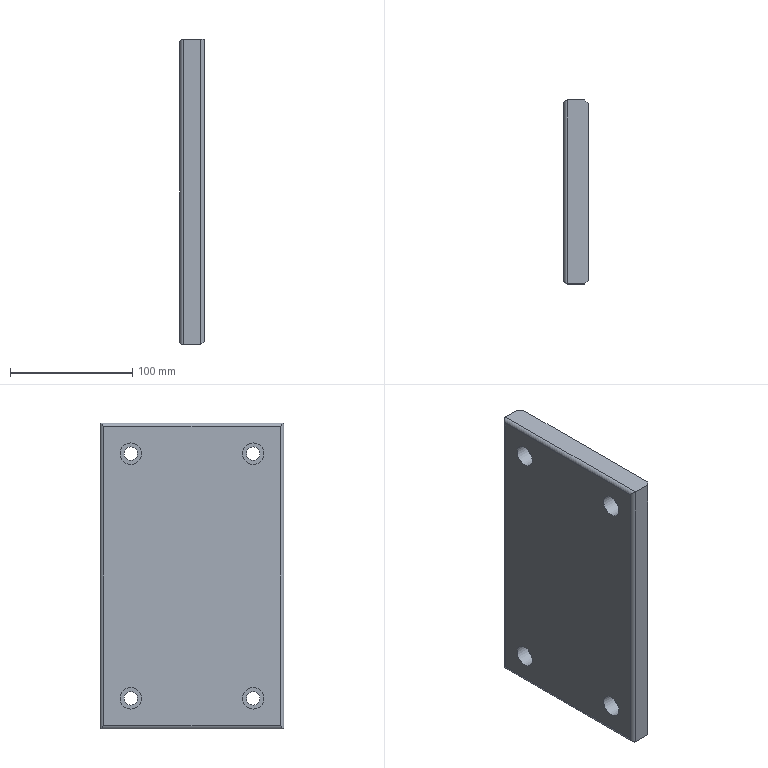Part | NX | features solid 2 | 1 solid | 25 faces | box 20 x 150 x 250 mm | volume 730972 mm3 | plane 13 | cylinder 12 | commonest cylinder face diameters 6 x4 11 x4 17.5 x4
STEP:
#1=CARTESIAN_POINT('',(-1123.,1070.,-255.));
#2=VERTEX_POINT('',#1);
#3=CARTESIAN_POINT('',(-1137.,1070.,-255.));
#4=VERTEX_POINT('',#3);
#5=CARTESIAN_POINT('',(-1120.,1070.,-255.));
#6=DIRECTION('',(-1.,0.,0.));
#7=VECTOR('',#6,1000.);
#8=LINE('',#5,#7);
#9=EDGE_CURVE('',#2,#4,#8,.T.);
#10=ORIENTED_EDGE('',*,*,#9,.F.);
#11=CARTESIAN_POINT('',(-1123.,920.,-255.));
#12=VERTEX_POINT('',#11);
#13=CARTESIAN_POINT('',(-1123.,920.,-255.));
#14=DIRECTION('',(0.,-1.,0.));
#15=VECTOR('',#14,1000.);
#16=LINE('',#13,#15);
#17=EDGE_CURVE('',#2,#12,#16,.T.);
#18=ORIENTED_EDGE('',*,*,#17,.T.);
#19=CARTESIAN_POINT('',(-1137.,920.,-255.));
#20=VERTEX_POINT('',#19);
#21=CARTESIAN_POINT('',(-1120.,920.,-255.));
#22=DIRECTION('',(-1.,0.,0.));
#23=VECTOR('',#22,1000.);
#24=LINE('',#21,#23);
#25=EDGE_CURVE('',#12,#20,#24,.T.);
#26=ORIENTED_EDGE('',*,*,#25,.T.);
#27=CARTESIAN_POINT('',(-1137.,1070.,-255.));
#28=DIRECTION('',(0.,1.,0.));
#29=VECTOR('',#28,1000.);
#30=LINE('',#27,#29);
#31=EDGE_CURVE('',#20,#4,#30,.T.);
#32=ORIENTED_EDGE('',*,*,#31,.T.);
#33=EDGE_LOOP('',(#10,#18,#26,#32));
#34=FACE_BOUND('',#33,.T.);
#35=CARTESIAN_POINT('',(-1120.,920.,-255.));
#36=DIRECTION('',(0.,0.,1.));
#37=DIRECTION('',(0.,-1.,0.));
#38=AXIS2_PLACEMENT_3D('',#35,#36,#37);
#39=PLANE('',#38);
#40=ADVANCED_FACE('',(#34),#39,.F.);
#41=CARTESIAN_POINT('',(-1123.,1070.,-5.));
#42=VERTEX_POINT('',#41);
#43=CARTESIAN_POINT('',(-1137.,1070.,-5.));
#44=VERTEX_POINT('',#43);
#45=CARTESIAN_POINT('',(-1120.,1070.,-5.));
#46=DIRECTION('',(-1.,0.,0.));
#47=VECTOR('',#46,1000.);
#48=LINE('',#45,#47);
#49=EDGE_CURVE('',#42,#44,#48,.T.);
#50=ORIENTED_EDGE('',*,*,#49,.F.);
#51=CARTESIAN_POINT('',(-1123.,1070.,-205.));
#52=DIRECTION('',(0.,0.,-1.));
#53=VECTOR('',#52,1000.);
#54=LINE('',#51,#53);
#55=EDGE_CURVE('',#42,#2,#54,.T.);
#56=ORIENTED_EDGE('',*,*,#55,.T.);
#57=ORIENTED_EDGE('',*,*,#9,.T.);
#58=CARTESIAN_POINT('',(-1137.,1070.,-5.));
#59=DIRECTION('',(0.,0.,1.));
#60=VECTOR('',#59,1000.);
#61=LINE('',#58,#60);
#62=EDGE_CURVE('',#4,#44,#61,.T.);
#63=ORIENTED_EDGE('',*,*,#62,.T.);
#64=EDGE_LOOP('',(#50,#56,#57,#63));
#65=FACE_BOUND('',#64,.T.);
#66=CARTESIAN_POINT('',(-1120.,1070.,-205.));
#67=DIRECTION('',(0.,-1.,0.));
#68=DIRECTION('',(1.,0.,0.));
#69=AXIS2_PLACEMENT_3D('',#66,#67,#68);
#70=PLANE('',#69);
#71=ADVANCED_FACE('',(#65),#70,.F.);
#72=CARTESIAN_POINT('',(-1123.,920.,-5.));
#73=VERTEX_POINT('',#72);
#74=CARTESIAN_POINT('',(-1137.,920.,-5.));
#75=VERTEX_POINT('',#74);
#76=CARTESIAN_POINT('',(-1120.,920.,-5.));
#77=DIRECTION('',(-1.,0.,0.));
#78=VECTOR('',#77,1000.);
#79=LINE('',#76,#78);
#80=EDGE_CURVE('',#73,#75,#79,.T.);
#81=ORIENTED_EDGE('',*,*,#80,.F.);
#82=CARTESIAN_POINT('',(-1120.,923.,-5.));
#83=VERTEX_POINT('',#82);
#84=CARTESIAN_POINT('',(-1120.,923.,-5.));
#85=DIRECTION('',(0.7071,0.7071,0.));
#86=VECTOR('',#85,1000.);
#87=LINE('',#84,#86);
#88=EDGE_CURVE('',#73,#83,#87,.T.);
#89=ORIENTED_EDGE('',*,*,#88,.T.);
#90=CARTESIAN_POINT('',(-1120.,1067.,-5.));
#91=VERTEX_POINT('',#90);
#92=CARTESIAN_POINT('',(-1120.,1070.,-5.));
#93=DIRECTION('',(0.,-1.,0.));
#94=VECTOR('',#93,1000.);
#95=LINE('',#92,#94);
#96=EDGE_CURVE('',#91,#83,#95,.T.);
#97=ORIENTED_EDGE('',*,*,#96,.F.);
#98=CARTESIAN_POINT('',(-1120.,1067.,-5.));
#99=DIRECTION('',(-0.7071,0.7071,0.));
#100=VECTOR('',#99,1000.);
#101=LINE('',#98,#100);
#102=EDGE_CURVE('',#91,#42,#101,.T.);
#103=ORIENTED_EDGE('',*,*,#102,.T.);
#104=ORIENTED_EDGE('',*,*,#49,.T.);
#105=CARTESIAN_POINT('',(-1137.,920.,-5.));
#106=DIRECTION('',(0.,-1.,0.));
#107=VECTOR('',#106,1000.);
#108=LINE('',#105,#107);
#109=EDGE_CURVE('',#44,#75,#108,.T.);
#110=ORIENTED_EDGE('',*,*,#109,.T.);
#111=EDGE_LOOP('',(#81,#89,#97,#103,#104,#110));
#112=FACE_BOUND('',#111,.T.);
#113=CARTESIAN_POINT('',(-1120.,1070.,-5.));
#114=DIRECTION('',(0.,0.,-1.));
#115=DIRECTION('',(1.,0.,0.));
#116=AXIS2_PLACEMENT_3D('',#113,#114,#115);
#117=PLANE('',#116);
#118=ADVANCED_FACE('',(#112),#117,.F.);
#119=ORIENTED_EDGE('',*,*,#25,.F.);
#120=CARTESIAN_POINT('',(-1123.,920.,-5.));
#121=DIRECTION('',(0.,0.,1.));
#122=VECTOR('',#121,1000.);
#123=LINE('',#120,#122);
#124=EDGE_CURVE('',#12,#73,#123,.T.);
#125=ORIENTED_EDGE('',*,*,#124,.T.);
#126=ORIENTED_EDGE('',*,*,#80,.T.);
#127=CARTESIAN_POINT('',(-1137.,920.,-205.));
#128=DIRECTION('',(0.,0.,-1.));
#129=VECTOR('',#128,1000.);
#130=LINE('',#127,#129);
#131=EDGE_CURVE('',#75,#20,#130,.T.);
#132=ORIENTED_EDGE('',*,*,#131,.T.);
#133=EDGE_LOOP('',(#119,#125,#126,#132));
#134=FACE_BOUND('',#133,.T.);
#135=CARTESIAN_POINT('',(-1120.,920.,-5.));
#136=DIRECTION('',(0.,1.,0.));
#137=DIRECTION('',(0.,0.,1.));
#138=AXIS2_PLACEMENT_3D('',#135,#136,#137);
#139=PLANE('',#138);
#140=ADVANCED_FACE('',(#134),#139,.F.);
#141=CARTESIAN_POINT('',(-1120.,1067.,-252.));
#142=VERTEX_POINT('',#141);
#143=CARTESIAN_POINT('',(-1120.,1067.,-205.));
#144=DIRECTION('',(0.,0.,1.));
#145=VECTOR('',#144,1000.);
#146=LINE('',#143,#145);
#147=EDGE_CURVE('',#142,#91,#146,.T.);
#148=ORIENTED_EDGE('',*,*,#147,.T.);
#149=ORIENTED_EDGE('',*,*,#96,.T.);
#150=CARTESIAN_POINT('',(-1120.,923.,-252.));
#151=VERTEX_POINT('',#150);
#152=CARTESIAN_POINT('',(-1120.,923.,-205.));
#153=DIRECTION('',(0.,0.,-1.));
#154=VECTOR('',#153,1000.);
#155=LINE('',#152,#154);
#156=EDGE_CURVE('',#83,#151,#155,.T.);
#157=ORIENTED_EDGE('',*,*,#156,.T.);
#158=CARTESIAN_POINT('',(-1120.,920.,-252.));
#159=DIRECTION('',(0.,1.,0.));
#160=VECTOR('',#159,1000.);
#161=LINE('',#158,#160);
#162=EDGE_CURVE('',#151,#142,#161,.T.);
#163=ORIENTED_EDGE('',*,*,#162,.T.);
#164=EDGE_LOOP('',(#148,#149,#157,#163));
#165=FACE_BOUND('',#164,.T.);
#166=CARTESIAN_POINT('',(-1120.,1045.,-35.5));
#167=VERTEX_POINT('',#166);
#168=CARTESIAN_POINT('',(-1120.,1045.,-30.));
#169=DIRECTION('',(-1.,0.,0.));
#170=DIRECTION('',(0.,0.,-1.));
#171=AXIS2_PLACEMENT_3D('',#168,#169,#170);
#172=CIRCLE('',#171,5.5);
#173=EDGE_CURVE('',#167,#167,#172,.T.);
#174=ORIENTED_EDGE('',*,*,#173,.T.);
#175=EDGE_LOOP('',(#174));
#176=FACE_BOUND('',#175,.T.);
#177=CARTESIAN_POINT('',(-1120.,945.,-35.5));
#178=VERTEX_POINT('',#177);
#179=CARTESIAN_POINT('',(-1120.,945.,-30.));
#180=DIRECTION('',(-1.,0.,0.));
#181=DIRECTION('',(0.,0.,-1.));
#182=AXIS2_PLACEMENT_3D('',#179,#180,#181);
#183=CIRCLE('',#182,5.5);
#184=EDGE_CURVE('',#178,#178,#183,.T.);
#185=ORIENTED_EDGE('',*,*,#184,.T.);
#186=EDGE_LOOP('',(#185));
#187=FACE_BOUND('',#186,.T.);
#188=CARTESIAN_POINT('',(-1120.,1045.,-235.5));
#189=VERTEX_POINT('',#188);
#190=CARTESIAN_POINT('',(-1120.,1045.,-230.));
#191=DIRECTION('',(-1.,0.,0.));
#192=DIRECTION('',(0.,0.,-1.));
#193=AXIS2_PLACEMENT_3D('',#190,#191,#192);
#194=CIRCLE('',#193,5.5);
#195=EDGE_CURVE('',#189,#189,#194,.T.);
#196=ORIENTED_EDGE('',*,*,#195,.T.);
#197=EDGE_LOOP('',(#196));
#198=FACE_BOUND('',#197,.T.);
#199=CARTESIAN_POINT('',(-1120.,945.,-235.5));
#200=VERTEX_POINT('',#199);
#201=CARTESIAN_POINT('',(-1120.,945.,-230.));
#202=DIRECTION('',(-1.,0.,0.));
#203=DIRECTION('',(0.,0.,-1.));
#204=AXIS2_PLACEMENT_3D('',#201,#202,#203);
#205=CIRCLE('',#204,5.5);
#206=EDGE_CURVE('',#200,#200,#205,.T.);
#207=ORIENTED_EDGE('',*,*,#206,.T.);
#208=EDGE_LOOP('',(#207));
#209=FACE_BOUND('',#208,.T.);
#210=CARTESIAN_POINT('',(-1120.,920.,-205.));
#211=DIRECTION('',(-1.,0.,0.));
#212=DIRECTION('',(0.,0.,-1.));
#213=AXIS2_PLACEMENT_3D('',#210,#211,#212);
#214=PLANE('',#213);
#215=ADVANCED_FACE('',(#165,#176,#187,#198,#209),#214,.F.);
#216=CARTESIAN_POINT('',(-1140.,1067.,-252.));
#217=VERTEX_POINT('',#216);
#218=CARTESIAN_POINT('',(-1140.,923.,-252.));
#219=VERTEX_POINT('',#218);
#220=CARTESIAN_POINT('',(-1140.,920.,-252.));
#221=DIRECTION('',(0.,1.,0.));
#222=VECTOR('',#221,1000.);
#223=LINE('',#220,#222);
#224=EDGE_CURVE('',#217,#219,#223,.F.);
#225=ORIENTED_EDGE('',*,*,#224,.T.);
#226=CARTESIAN_POINT('',(-1140.,923.,-8.));
#227=VERTEX_POINT('',#226);
#228=CARTESIAN_POINT('',(-1140.,923.,-5.));
#229=DIRECTION('',(0.,0.,-1.));
#230=VECTOR('',#229,1000.);
#231=LINE('',#228,#230);
#232=EDGE_CURVE('',#219,#227,#231,.F.);
#233=ORIENTED_EDGE('',*,*,#232,.T.);
#234=CARTESIAN_POINT('',(-1140.,1067.,-8.));
#235=VERTEX_POINT('',#234);
#236=CARTESIAN_POINT('',(-1140.,1070.,-8.));
#237=DIRECTION('',(0.,-1.,0.));
#238=VECTOR('',#237,1000.);
#239=LINE('',#236,#238);
#240=EDGE_CURVE('',#227,#235,#239,.F.);
#241=ORIENTED_EDGE('',*,*,#240,.T.);
#242=CARTESIAN_POINT('',(-1140.,1067.,-205.));
#243=DIRECTION('',(0.,0.,1.));
#244=VECTOR('',#243,1000.);
#245=LINE('',#242,#244);
#246=EDGE_CURVE('',#235,#217,#245,.F.);
#247=ORIENTED_EDGE('',*,*,#246,.T.);
#248=EDGE_LOOP('',(#225,#233,#241,#247));
#249=FACE_BOUND('',#248,.T.);
#250=CARTESIAN_POINT('',(-1140.,1045.,-21.25));
#251=VERTEX_POINT('',#250);
#252=CARTESIAN_POINT('',(-1140.,1045.,-30.));
#253=DIRECTION('',(1.,0.,0.));
#254=DIRECTION('',(0.,0.,1.));
#255=AXIS2_PLACEMENT_3D('',#252,#253,#254);
#256=CIRCLE('',#255,8.75);
#257=EDGE_CURVE('',#251,#251,#256,.T.);
#258=ORIENTED_EDGE('',*,*,#257,.T.);
#259=EDGE_LOOP('',(#258));
#260=FACE_BOUND('',#259,.T.);
#261=CARTESIAN_POINT('',(-1140.,945.,-21.25));
#262=VERTEX_POINT('',#261);
#263=CARTESIAN_POINT('',(-1140.,945.,-30.));
#264=DIRECTION('',(1.,0.,0.));
#265=DIRECTION('',(0.,0.,1.));
#266=AXIS2_PLACEMENT_3D('',#263,#264,#265);
#267=CIRCLE('',#266,8.75);
#268=EDGE_CURVE('',#262,#262,#267,.T.);
#269=ORIENTED_EDGE('',*,*,#268,.T.);
#270=EDGE_LOOP('',(#269));
#271=FACE_BOUND('',#270,.T.);
#272=CARTESIAN_POINT('',(-1140.,1045.,-221.25));
#273=VERTEX_POINT('',#272);
#274=CARTESIAN_POINT('',(-1140.,1045.,-230.));
#275=DIRECTION('',(1.,0.,0.));
#276=DIRECTION('',(0.,0.,1.));
#277=AXIS2_PLACEMENT_3D('',#274,#275,#276);
#278=CIRCLE('',#277,8.75);
#279=EDGE_CURVE('',#273,#273,#278,.T.);
#280=ORIENTED_EDGE('',*,*,#279,.T.);
#281=EDGE_LOOP('',(#280));
#282=FACE_BOUND('',#281,.T.);
#283=CARTESIAN_POINT('',(-1140.,945.,-221.25));
#284=VERTEX_POINT('',#283);
#285=CARTESIAN_POINT('',(-1140.,945.,-230.));
#286=DIRECTION('',(1.,0.,0.));
#287=DIRECTION('',(0.,0.,1.));
#288=AXIS2_PLACEMENT_3D('',#285,#286,#287);
#289=CIRCLE('',#288,8.75);
#290=EDGE_CURVE('',#284,#284,#289,.T.);
#291=ORIENTED_EDGE('',*,*,#290,.T.);
#292=EDGE_LOOP('',(#291));
#293=FACE_BOUND('',#292,.T.);
#294=CARTESIAN_POINT('',(-1140.,920.,-205.));
#295=DIRECTION('',(-1.,0.,0.));
#296=DIRECTION('',(0.,0.,-1.));
#297=AXIS2_PLACEMENT_3D('',#294,#295,#296);
#298=PLANE('',#297);
#299=ADVANCED_FACE('',(#249,#260,#271,#282,#293),#298,.T.);
#300=CARTESIAN_POINT('',(-1128.,945.,-224.5));
#301=VERTEX_POINT('',#300);
#302=CARTESIAN_POINT('',(-1128.,945.,-230.));
#303=DIRECTION('',(1.,0.,0.));
#304=DIRECTION('',(0.,0.,1.));
#305=AXIS2_PLACEMENT_3D('',#302,#303,#304);
#306=CIRCLE('',#305,5.5);
#307=EDGE_CURVE('',#301,#301,#306,.T.);
#308=ORIENTED_EDGE('',*,*,#307,.F.);
#309=EDGE_LOOP('',(#308));
#310=FACE_BOUND('',#309,.T.);
#311=ORIENTED_EDGE('',*,*,#206,.F.);
#312=EDGE_LOOP('',(#311));
#313=FACE_BOUND('',#312,.T.);
#314=CARTESIAN_POINT('',(-1090.,945.,-230.));
#315=DIRECTION('',(1.,0.,0.));
#316=DIRECTION('',(0.,0.,1.));
#317=AXIS2_PLACEMENT_3D('',#314,#315,#316);
#318=CYLINDRICAL_SURFACE('',#317,5.5);
#319=ADVANCED_FACE('',(#310,#313),#318,.F.);
#320=ORIENTED_EDGE('',*,*,#307,.T.);
#321=EDGE_LOOP('',(#320));
#322=FACE_BOUND('',#321,.T.);
#323=CARTESIAN_POINT('',(-1128.,945.,-221.25));
#324=VERTEX_POINT('',#323);
#325=CARTESIAN_POINT('',(-1128.,945.,-230.));
#326=DIRECTION('',(1.,0.,0.));
#327=DIRECTION('',(0.,0.,1.));
#328=AXIS2_PLACEMENT_3D('',#325,#326,#327);
#329=CIRCLE('',#328,8.75);
#330=EDGE_CURVE('',#324,#324,#329,.T.);
#331=ORIENTED_EDGE('',*,*,#330,.F.);
#332=EDGE_LOOP('',(#331));
#333=FACE_BOUND('',#332,.T.);
#334=CARTESIAN_POINT('',(-1128.,945.,-230.));
#335=DIRECTION('',(1.,0.,0.));
#336=DIRECTION('',(0.,0.,1.));
#337=AXIS2_PLACEMENT_3D('',#334,#335,#336);
#338=PLANE('',#337);
#339=ADVANCED_FACE('',(#322,#333),#338,.F.);
#340=ORIENTED_EDGE('',*,*,#330,.T.);
#341=EDGE_LOOP('',(#340));
#342=FACE_BOUND('',#341,.T.);
#343=ORIENTED_EDGE('',*,*,#290,.F.);
#344=EDGE_LOOP('',(#343));
#345=FACE_BOUND('',#344,.T.);
#346=CARTESIAN_POINT('',(-1140.,945.,-230.));
#347=DIRECTION('',(1.,0.,0.));
#348=DIRECTION('',(0.,0.,1.));
#349=AXIS2_PLACEMENT_3D('',#346,#347,#348);
#350=CYLINDRICAL_SURFACE('',#349,8.75);
#351=ADVANCED_FACE('',(#342,#345),#350,.F.);
#352=CARTESIAN_POINT('',(-1128.,1045.,-224.5));
#353=VERTEX_POINT('',#352);
#354=CARTESIAN_POINT('',(-1128.,1045.,-230.));
#355=DIRECTION('',(1.,0.,0.));
#356=DIRECTION('',(0.,0.,1.));
#357=AXIS2_PLACEMENT_3D('',#354,#355,#356);
#358=CIRCLE('',#357,5.5);
#359=EDGE_CURVE('',#353,#353,#358,.T.);
#360=ORIENTED_EDGE('',*,*,#359,.F.);
#361=EDGE_LOOP('',(#360));
#362=FACE_BOUND('',#361,.T.);
#363=ORIENTED_EDGE('',*,*,#195,.F.);
#364=EDGE_LOOP('',(#363));
#365=FACE_BOUND('',#364,.T.);
#366=CARTESIAN_POINT('',(-1090.,1045.,-230.));
#367=DIRECTION('',(1.,0.,0.));
#368=DIRECTION('',(0.,0.,1.));
#369=AXIS2_PLACEMENT_3D('',#366,#367,#368);
#370=CYLINDRICAL_SURFACE('',#369,5.5);
#371=ADVANCED_FACE('',(#362,#365),#370,.F.);
#372=ORIENTED_EDGE('',*,*,#359,.T.);
#373=EDGE_LOOP('',(#372));
#374=FACE_BOUND('',#373,.T.);
#375=CARTESIAN_POINT('',(-1128.,1045.,-221.25));
#376=VERTEX_POINT('',#375);
#377=CARTESIAN_POINT('',(-1128.,1045.,-230.));
#378=DIRECTION('',(1.,0.,0.));
#379=DIRECTION('',(0.,0.,1.));
#380=AXIS2_PLACEMENT_3D('',#377,#378,#379);
#381=CIRCLE('',#380,8.75);
#382=EDGE_CURVE('',#376,#376,#381,.T.);
#383=ORIENTED_EDGE('',*,*,#382,.F.);
#384=EDGE_LOOP('',(#383));
#385=FACE_BOUND('',#384,.T.);
#386=CARTESIAN_POINT('',(-1128.,1045.,-230.));
#387=DIRECTION('',(1.,0.,0.));
#388=DIRECTION('',(0.,0.,1.));
#389=AXIS2_PLACEMENT_3D('',#386,#387,#388);
#390=PLANE('',#389);
#391=ADVANCED_FACE('',(#374,#385),#390,.F.);
#392=ORIENTED_EDGE('',*,*,#382,.T.);
#393=EDGE_LOOP('',(#392));
#394=FACE_BOUND('',#393,.T.);
#395=ORIENTED_EDGE('',*,*,#279,.F.);
#396=EDGE_LOOP('',(#395));
#397=FACE_BOUND('',#396,.T.);
#398=CARTESIAN_POINT('',(-1140.,1045.,-230.));
#399=DIRECTION('',(1.,0.,0.));
#400=DIRECTION('',(0.,0.,1.));
#401=AXIS2_PLACEMENT_3D('',#398,#399,#400);
#402=CYLINDRICAL_SURFACE('',#401,8.75);
#403=ADVANCED_FACE('',(#394,#397),#402,.F.);
#404=CARTESIAN_POINT('',(-1128.,945.,-24.5));
#405=VERTEX_POINT('',#404);
#406=CARTESIAN_POINT('',(-1128.,945.,-30.));
#407=DIRECTION('',(1.,0.,0.));
#408=DIRECTION('',(0.,0.,1.));
#409=AXIS2_PLACEMENT_3D('',#406,#407,#408);
#410=CIRCLE('',#409,5.5);
#411=EDGE_CURVE('',#405,#405,#410,.T.);
#412=ORIENTED_EDGE('',*,*,#411,.F.);
#413=EDGE_LOOP('',(#412));
#414=FACE_BOUND('',#413,.T.);
#415=ORIENTED_EDGE('',*,*,#184,.F.);
#416=EDGE_LOOP('',(#415));
#417=FACE_BOUND('',#416,.T.);
#418=CARTESIAN_POINT('',(-1090.,945.,-30.));
#419=DIRECTION('',(1.,0.,0.));
#420=DIRECTION('',(0.,0.,1.));
#421=AXIS2_PLACEMENT_3D('',#418,#419,#420);
#422=CYLINDRICAL_SURFACE('',#421,5.5);
#423=ADVANCED_FACE('',(#414,#417),#422,.F.);
#424=ORIENTED_EDGE('',*,*,#411,.T.);
#425=EDGE_LOOP('',(#424));
#426=FACE_BOUND('',#425,.T.);
#427=CARTESIAN_POINT('',(-1128.,945.,-21.25));
#428=VERTEX_POINT('',#427);
#429=CARTESIAN_POINT('',(-1128.,945.,-30.));
#430=DIRECTION('',(1.,0.,0.));
#431=DIRECTION('',(0.,0.,1.));
#432=AXIS2_PLACEMENT_3D('',#429,#430,#431);
#433=CIRCLE('',#432,8.75);
#434=EDGE_CURVE('',#428,#428,#433,.T.);
#435=ORIENTED_EDGE('',*,*,#434,.F.);
#436=EDGE_LOOP('',(#435));
#437=FACE_BOUND('',#436,.T.);
#438=CARTESIAN_POINT('',(-1128.,945.,-30.));
#439=DIRECTION('',(1.,0.,0.));
#440=DIRECTION('',(0.,0.,1.));
#441=AXIS2_PLACEMENT_3D('',#438,#439,#440);
#442=PLANE('',#441);
#443=ADVANCED_FACE('',(#426,#437),#442,.F.);
#444=ORIENTED_EDGE('',*,*,#434,.T.);
#445=EDGE_LOOP('',(#444));
#446=FACE_BOUND('',#445,.T.);
#447=ORIENTED_EDGE('',*,*,#268,.F.);
#448=EDGE_LOOP('',(#447));
#449=FACE_BOUND('',#448,.T.);
#450=CARTESIAN_POINT('',(-1140.,945.,-30.));
#451=DIRECTION('',(1.,0.,0.));
#452=DIRECTION('',(0.,0.,1.));
#453=AXIS2_PLACEMENT_3D('',#450,#451,#452);
#454=CYLINDRICAL_SURFACE('',#453,8.75);
#455=ADVANCED_FACE('',(#446,#449),#454,.F.);
#456=CARTESIAN_POINT('',(-1128.,1045.,-24.5));
#457=VERTEX_POINT('',#456);
#458=CARTESIAN_POINT('',(-1128.,1045.,-30.));
#459=DIRECTION('',(1.,0.,0.));
#460=DIRECTION('',(0.,0.,1.));
#461=AXIS2_PLACEMENT_3D('',#458,#459,#460);
#462=CIRCLE('',#461,5.5);
#463=EDGE_CURVE('',#457,#457,#462,.T.);
#464=ORIENTED_EDGE('',*,*,#463,.F.);
#465=EDGE_LOOP('',(#464));
#466=FACE_BOUND('',#465,.T.);
#467=ORIENTED_EDGE('',*,*,#173,.F.);
#468=EDGE_LOOP('',(#467));
#469=FACE_BOUND('',#468,.T.);
#470=CARTESIAN_POINT('',(-1090.,1045.,-30.));
#471=DIRECTION('',(1.,0.,0.));
#472=DIRECTION('',(0.,0.,1.));
#473=AXIS2_PLACEMENT_3D('',#470,#471,#472);
#474=CYLINDRICAL_SURFACE('',#473,5.5);
#475=ADVANCED_FACE('',(#466,#469),#474,.F.);
#476=ORIENTED_EDGE('',*,*,#463,.T.);
#477=EDGE_LOOP('',(#476));
#478=FACE_BOUND('',#477,.T.);
#479=CARTESIAN_POINT('',(-1128.,1045.,-21.25));
#480=VERTEX_POINT('',#479);
#481=CARTESIAN_POINT('',(-1128.,1045.,-30.));
#482=DIRECTION('',(1.,0.,0.));
#483=DIRECTION('',(0.,0.,1.));
#484=AXIS2_PLACEMENT_3D('',#481,#482,#483);
#485=CIRCLE('',#484,8.75);
#486=EDGE_CURVE('',#480,#480,#485,.T.);
#487=ORIENTED_EDGE('',*,*,#486,.F.);
#488=EDGE_LOOP('',(#487));
#489=FACE_BOUND('',#488,.T.);
#490=CARTESIAN_POINT('',(-1128.,1045.,-30.));
#491=DIRECTION('',(1.,0.,0.));
#492=DIRECTION('',(0.,0.,1.));
#493=AXIS2_PLACEMENT_3D('',#490,#491,#492);
#494=PLANE('',#493);
#495=ADVANCED_FACE('',(#478,#489),#494,.F.);
#496=ORIENTED_EDGE('',*,*,#486,.T.);
#497=EDGE_LOOP('',(#496));
#498=FACE_BOUND('',#497,.T.);
#499=ORIENTED_EDGE('',*,*,#257,.F.);
#500=EDGE_LOOP('',(#499));
#501=FACE_BOUND('',#500,.T.);
#502=CARTESIAN_POINT('',(-1140.,1045.,-30.));
#503=DIRECTION('',(1.,0.,0.));
#504=DIRECTION('',(0.,0.,1.));
#505=AXIS2_PLACEMENT_3D('',#502,#503,#504);
#506=CYLINDRICAL_SURFACE('',#505,8.75);
#507=ADVANCED_FACE('',(#498,#501),#506,.F.);
#508=CARTESIAN_POINT('',(-1137.,1067.,-252.));
#509=DIRECTION('',(0.,-0.7071,-0.7071));
#510=DIRECTION('',(0.,-0.7071,0.7071));
#511=AXIS2_PLACEMENT_3D('',#508,#509,#510);
#512=ELLIPSE('',#511,4.243,3.);
#513=EDGE_CURVE('',#217,#4,#512,.T.);
#514=ORIENTED_EDGE('',*,*,#513,.F.);
#515=ORIENTED_EDGE('',*,*,#246,.F.);
#516=CARTESIAN_POINT('',(-1137.,1067.,-8.));
#517=DIRECTION('',(0.,0.7071,-0.7071));
#518=DIRECTION('',(0.,-0.7071,-0.7071));
#519=AXIS2_PLACEMENT_3D('',#516,#517,#518);
#520=ELLIPSE('',#519,4.243,3.);
#521=EDGE_CURVE('',#44,#235,#520,.F.);
#522=ORIENTED_EDGE('',*,*,#521,.F.);
#523=ORIENTED_EDGE('',*,*,#62,.F.);
#524=EDGE_LOOP('',(#514,#515,#522,#523));
#525=FACE_BOUND('',#524,.T.);
#526=CARTESIAN_POINT('',(-1137.,1067.,-205.));
#527=DIRECTION('',(0.,0.,-1.));
#528=DIRECTION('',(1.,0.,0.));
#529=AXIS2_PLACEMENT_3D('',#526,#527,#528);
#530=CYLINDRICAL_SURFACE('',#529,3.);
#531=ADVANCED_FACE('',(#525),#530,.T.);
#532=ORIENTED_EDGE('',*,*,#521,.T.);
#533=ORIENTED_EDGE('',*,*,#240,.F.);
#534=CARTESIAN_POINT('',(-1137.,923.,-8.));
#535=DIRECTION('',(0.,0.7071,0.7071));
#536=DIRECTION('',(0.,0.7071,-0.7071));
#537=AXIS2_PLACEMENT_3D('',#534,#535,#536);
#538=ELLIPSE('',#537,4.243,3.);
#539=EDGE_CURVE('',#75,#227,#538,.F.);
#540=ORIENTED_EDGE('',*,*,#539,.F.);
#541=ORIENTED_EDGE('',*,*,#109,.F.);
#542=EDGE_LOOP('',(#532,#533,#540,#541));
#543=FACE_BOUND('',#542,.T.);
#544=CARTESIAN_POINT('',(-1137.,1070.,-8.));
#545=DIRECTION('',(0.,1.,0.));
#546=DIRECTION('',(-1.,0.,0.));
#547=AXIS2_PLACEMENT_3D('',#544,#545,#546);
#548=CYLINDRICAL_SURFACE('',#547,3.);
#549=ADVANCED_FACE('',(#543),#548,.T.);
#550=ORIENTED_EDGE('',*,*,#513,.T.);
#551=ORIENTED_EDGE('',*,*,#31,.F.);
#552=CARTESIAN_POINT('',(-1137.,923.,-252.));
#553=DIRECTION('',(0.,-0.7071,0.7071));
#554=DIRECTION('',(0.,-0.7071,-0.7071));
#555=AXIS2_PLACEMENT_3D('',#552,#553,#554);
#556=ELLIPSE('',#555,4.243,3.);
#557=EDGE_CURVE('',#219,#20,#556,.T.);
#558=ORIENTED_EDGE('',*,*,#557,.F.);
#559=ORIENTED_EDGE('',*,*,#224,.F.);
#560=EDGE_LOOP('',(#550,#551,#558,#559));
#561=FACE_BOUND('',#560,.T.);
#562=CARTESIAN_POINT('',(-1137.,920.,-252.));
#563=DIRECTION('',(0.,-1.,0.));
#564=DIRECTION('',(0.,0.,-1.));
#565=AXIS2_PLACEMENT_3D('',#562,#563,#564);
#566=CYLINDRICAL_SURFACE('',#565,3.);
#567=ADVANCED_FACE('',(#561),#566,.T.);
#568=ORIENTED_EDGE('',*,*,#539,.T.);
#569=ORIENTED_EDGE('',*,*,#232,.F.);
#570=ORIENTED_EDGE('',*,*,#557,.T.);
#571=ORIENTED_EDGE('',*,*,#131,.F.);
#572=EDGE_LOOP('',(#568,#569,#570,#571));
#573=FACE_BOUND('',#572,.T.);
#574=CARTESIAN_POINT('',(-1137.,923.,-5.));
#575=DIRECTION('',(0.,0.,1.));
#576=DIRECTION('',(0.,-1.,0.));
#577=AXIS2_PLACEMENT_3D('',#574,#575,#576);
#578=CYLINDRICAL_SURFACE('',#577,3.);
#579=ADVANCED_FACE('',(#573),#578,.T.);
#580=CARTESIAN_POINT('',(-1121.,922.,-253.));
#581=DIRECTION('',(0.5774,0.5774,0.5774));
#582=VECTOR('',#581,1000.);
#583=LINE('',#580,#582);
#584=EDGE_CURVE('',#12,#151,#583,.T.);
#585=ORIENTED_EDGE('',*,*,#584,.F.);
#586=ORIENTED_EDGE('',*,*,#17,.F.);
#587=CARTESIAN_POINT('',(-1071.,1018.,-203.));
#588=DIRECTION('',(0.5774,-0.5774,0.5774));
#589=VECTOR('',#588,1000.);
#590=LINE('',#587,#589);
#591=EDGE_CURVE('',#142,#2,#590,.F.);
#592=ORIENTED_EDGE('',*,*,#591,.F.);
#593=ORIENTED_EDGE('',*,*,#162,.F.);
#594=EDGE_LOOP('',(#585,#586,#592,#593));
#595=FACE_BOUND('',#594,.T.);
#596=CARTESIAN_POINT('',(-1120.,920.,-252.));
#597=DIRECTION('',(-0.7071,0.,0.7071));
#598=DIRECTION('',(-0.7071,0.,-0.7071));
#599=AXIS2_PLACEMENT_3D('',#596,#597,#598);
#600=PLANE('',#599);
#601=ADVANCED_FACE('',(#595),#600,.F.);
#602=ORIENTED_EDGE('',*,*,#591,.T.);
#603=ORIENTED_EDGE('',*,*,#55,.F.);
#604=ORIENTED_EDGE('',*,*,#102,.F.);
#605=ORIENTED_EDGE('',*,*,#147,.F.);
#606=EDGE_LOOP('',(#602,#603,#604,#605));
#607=FACE_BOUND('',#606,.T.);
#608=CARTESIAN_POINT('',(-1120.,1067.,-205.));
#609=DIRECTION('',(-0.7071,-0.7071,0.));
#610=DIRECTION('',(0.7071,-0.7071,0.));
#611=AXIS2_PLACEMENT_3D('',#608,#609,#610);
#612=PLANE('',#611);
#613=ADVANCED_FACE('',(#607),#612,.F.);
#614=ORIENTED_EDGE('',*,*,#584,.T.);
#615=ORIENTED_EDGE('',*,*,#156,.F.);
#616=ORIENTED_EDGE('',*,*,#88,.F.);
#617=ORIENTED_EDGE('',*,*,#124,.F.);
#618=EDGE_LOOP('',(#614,#615,#616,#617));
#619=FACE_BOUND('',#618,.T.);
#620=CARTESIAN_POINT('',(-1120.,923.,-205.));
#621=DIRECTION('',(-0.7071,0.7071,0.));
#622=DIRECTION('',(-0.7071,-0.7071,0.));
#623=AXIS2_PLACEMENT_3D('',#620,#621,#622);
#624=PLANE('',#623);
#625=ADVANCED_FACE('',(#619),#624,.F.);
#626=CLOSED_SHELL('',(#40,#71,#118,#140,#215,#299,#319,#339,#351,#371,#391,#403,#423,#443,#455,#475,#495,#507,#531,#549,#567,#579,#601,#613,#625));
#627=MANIFOLD_SOLID_BREP('',#626);
#628=(LENGTH_UNIT()NAMED_UNIT(*)SI_UNIT(.MILLI.,.METRE.));
#629=UNCERTAINTY_MEASURE_WITH_UNIT(LENGTH_MEASURE(0.00001),#628,'','');
#630=(NAMED_UNIT(*)PLANE_ANGLE_UNIT()SI_UNIT($,.RADIAN.));
#631=(NAMED_UNIT(*)SI_UNIT($,.STERADIAN.)SOLID_ANGLE_UNIT());
#632=(GEOMETRIC_REPRESENTATION_CONTEXT(3)GLOBAL_UNCERTAINTY_ASSIGNED_CONTEXT((#629))GLOBAL_UNIT_ASSIGNED_CONTEXT((#628,#630,#631))REPRESENTATION_CONTEXT('',''));
#633=ADVANCED_BREP_SHAPE_REPRESENTATION('',(#627),#632);